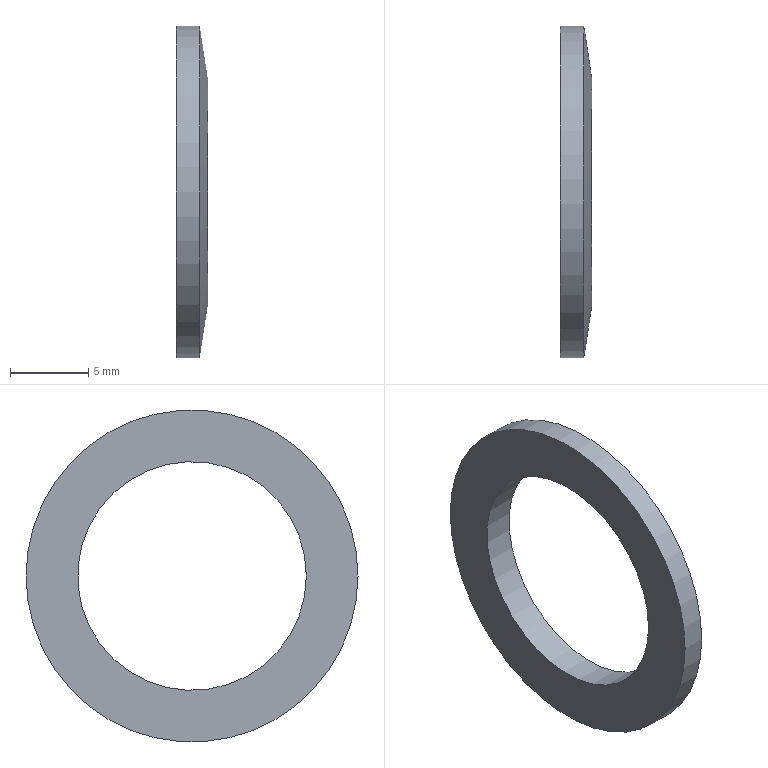Part | NX | features HZGN_5003_019_C-AC1412S 2 | 1 solid | 4 faces | box 2 x 21.2 x 21.2 mm | volume 321.903 mm3 | cylinder 2 | plane 1 | cone 1 | commonest cylinder face diameters 14.6 x1 21.2 x1
STEP:
#1=CARTESIAN_POINT('',(91.6,-147.6,-223.));
#2=VERTEX_POINT('',#1);
#3=CARTESIAN_POINT('',(91.6,-137.,-223.));
#4=DIRECTION('',(-1.,0.,0.));
#5=DIRECTION('',(0.,-1.,0.));
#6=AXIS2_PLACEMENT_3D('',#3,#4,#5);
#7=CIRCLE('',#6,10.6);
#8=EDGE_CURVE('',#2,#2,#7,.T.);
#9=ORIENTED_EDGE('',*,*,#8,.T.);
#10=EDGE_LOOP('',(#9));
#11=FACE_BOUND('',#10,.T.);
#12=CARTESIAN_POINT('',(90.1,-147.6,-223.));
#13=VERTEX_POINT('',#12);
#14=CARTESIAN_POINT('',(90.1,-137.,-223.));
#15=DIRECTION('',(-1.,0.,0.));
#16=DIRECTION('',(0.,-1.,0.));
#17=AXIS2_PLACEMENT_3D('',#14,#15,#16);
#18=CIRCLE('',#17,10.6);
#19=EDGE_CURVE('',#13,#13,#18,.T.);
#20=ORIENTED_EDGE('',*,*,#19,.F.);
#21=EDGE_LOOP('',(#20));
#22=FACE_BOUND('',#21,.T.);
#23=CARTESIAN_POINT('',(90.,-137.,-223.));
#24=DIRECTION('',(-1.,0.,0.));
#25=DIRECTION('',(0.,-1.,0.));
#26=AXIS2_PLACEMENT_3D('',#23,#24,#25);
#27=CYLINDRICAL_SURFACE('',#26,10.6);
#28=ADVANCED_FACE('',(#11,#22),#27,.T.);
#29=ORIENTED_EDGE('',*,*,#19,.T.);
#30=EDGE_LOOP('',(#29));
#31=FACE_BOUND('',#30,.T.);
#32=CARTESIAN_POINT('',(90.1,-144.3,-223.));
#33=VERTEX_POINT('',#32);
#34=CARTESIAN_POINT('',(90.1,-137.,-223.));
#35=DIRECTION('',(-1.,0.,0.));
#36=DIRECTION('',(0.,-1.,0.));
#37=AXIS2_PLACEMENT_3D('',#34,#35,#36);
#38=CIRCLE('',#37,7.3);
#39=EDGE_CURVE('',#33,#33,#38,.T.);
#40=ORIENTED_EDGE('',*,*,#39,.F.);
#41=EDGE_LOOP('',(#40));
#42=FACE_BOUND('',#41,.T.);
#43=CARTESIAN_POINT('',(90.1,-137.,-212.4));
#44=DIRECTION('',(-1.,0.,0.));
#45=DIRECTION('',(0.,-1.,0.));
#46=AXIS2_PLACEMENT_3D('',#43,#44,#45);
#47=PLANE('',#46);
#48=ADVANCED_FACE('',(#31,#42),#47,.T.);
#49=ORIENTED_EDGE('',*,*,#39,.T.);
#50=EDGE_LOOP('',(#49));
#51=FACE_BOUND('',#50,.T.);
#52=CARTESIAN_POINT('',(92.1,-144.3,-223.));
#53=VERTEX_POINT('',#52);
#54=CARTESIAN_POINT('',(92.1,-137.,-223.));
#55=DIRECTION('',(-1.,0.,0.));
#56=DIRECTION('',(0.,-1.,0.));
#57=AXIS2_PLACEMENT_3D('',#54,#55,#56);
#58=CIRCLE('',#57,7.3);
#59=EDGE_CURVE('',#53,#53,#58,.T.);
#60=ORIENTED_EDGE('',*,*,#59,.F.);
#61=EDGE_LOOP('',(#60));
#62=FACE_BOUND('',#61,.T.);
#63=CARTESIAN_POINT('',(90.,-137.,-223.));
#64=DIRECTION('',(-1.,0.,0.));
#65=DIRECTION('',(0.,-1.,0.));
#66=AXIS2_PLACEMENT_3D('',#63,#64,#65);
#67=CYLINDRICAL_SURFACE('',#66,7.3);
#68=ADVANCED_FACE('',(#51,#62),#67,.F.);
#69=ORIENTED_EDGE('',*,*,#59,.T.);
#70=EDGE_LOOP('',(#69));
#71=FACE_BOUND('',#70,.T.);
#72=ORIENTED_EDGE('',*,*,#8,.F.);
#73=EDGE_LOOP('',(#72));
#74=FACE_BOUND('',#73,.T.);
#75=CARTESIAN_POINT('',(91.6,-137.,-223.));
#76=DIRECTION('',(-1.,0.,0.));
#77=DIRECTION('',(0.,-1.,0.));
#78=AXIS2_PLACEMENT_3D('',#75,#76,#77);
#79=CONICAL_SURFACE('',#78,10.6,1.42);
#80=ADVANCED_FACE('',(#71,#74),#79,.T.);
#81=CLOSED_SHELL('',(#28,#48,#68,#80));
#82=MANIFOLD_SOLID_BREP('',#81);
#83=(LENGTH_UNIT()NAMED_UNIT(*)SI_UNIT(.MILLI.,.METRE.));
#84=UNCERTAINTY_MEASURE_WITH_UNIT(LENGTH_MEASURE(0.00001),#83,'','');
#85=(NAMED_UNIT(*)PLANE_ANGLE_UNIT()SI_UNIT($,.RADIAN.));
#86=(NAMED_UNIT(*)SI_UNIT($,.STERADIAN.)SOLID_ANGLE_UNIT());
#87=(GEOMETRIC_REPRESENTATION_CONTEXT(3)GLOBAL_UNCERTAINTY_ASSIGNED_CONTEXT((#84))GLOBAL_UNIT_ASSIGNED_CONTEXT((#83,#85,#86))REPRESENTATION_CONTEXT('',''));
#88=ADVANCED_BREP_SHAPE_REPRESENTATION('',(#82),#87);